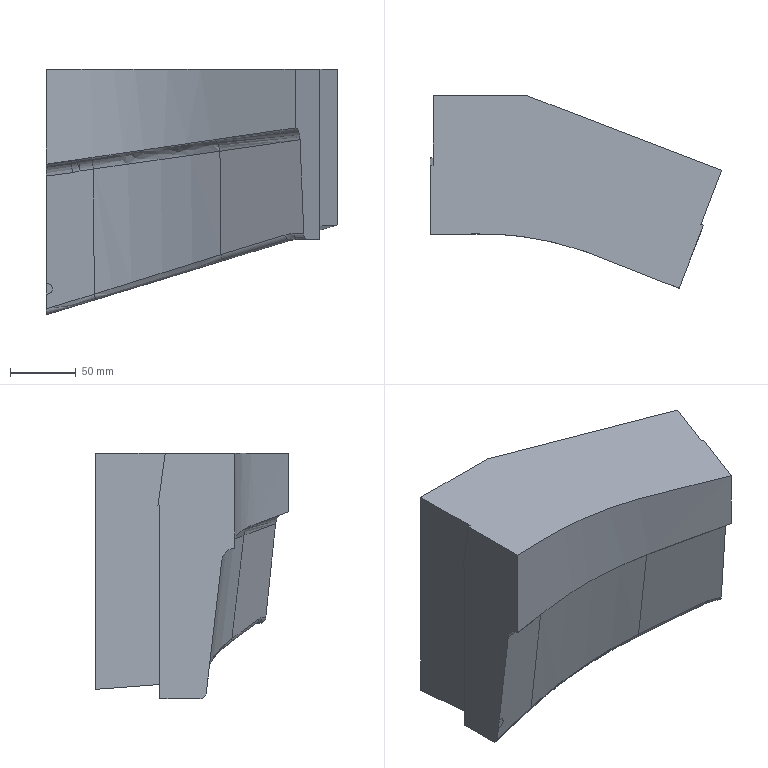Part | NX | features solid 2 | 1 solid | 36 faces | box 222.159 x 147.058 x 187.35 mm | volume 2987798 mm3 | spline 23 | plane 13